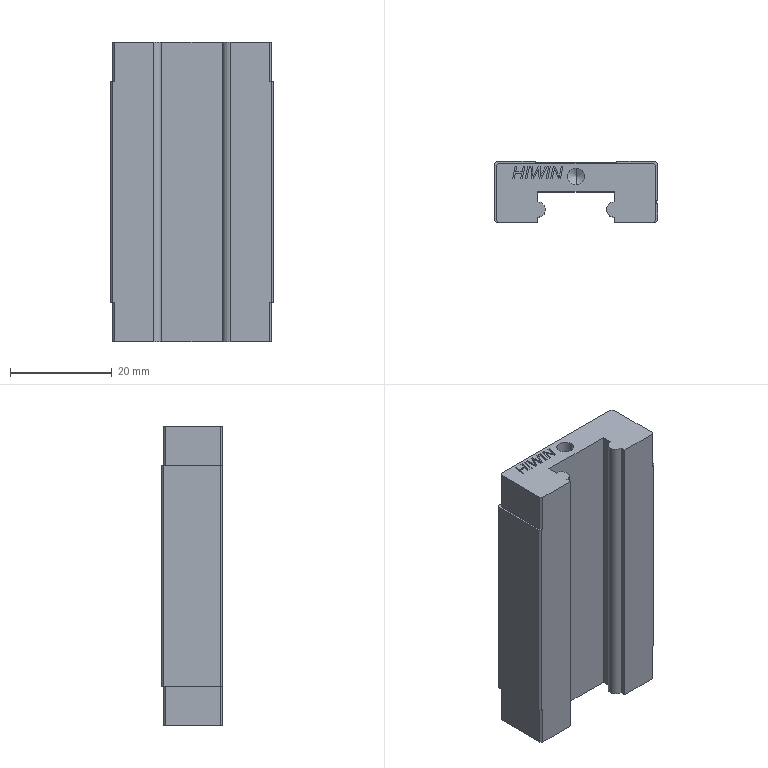Part | SolidWorks | features BaseBody 5 | 5 solids | 251 faces | box 32 x 12 x 58.8 mm | volume 16967 mm3 | plane 141 | cylinder 41 | spline 40 | cone 29 | commonest cylinder face diameters 3 x19 2.5 x16 3.3 x4 0.6 x2